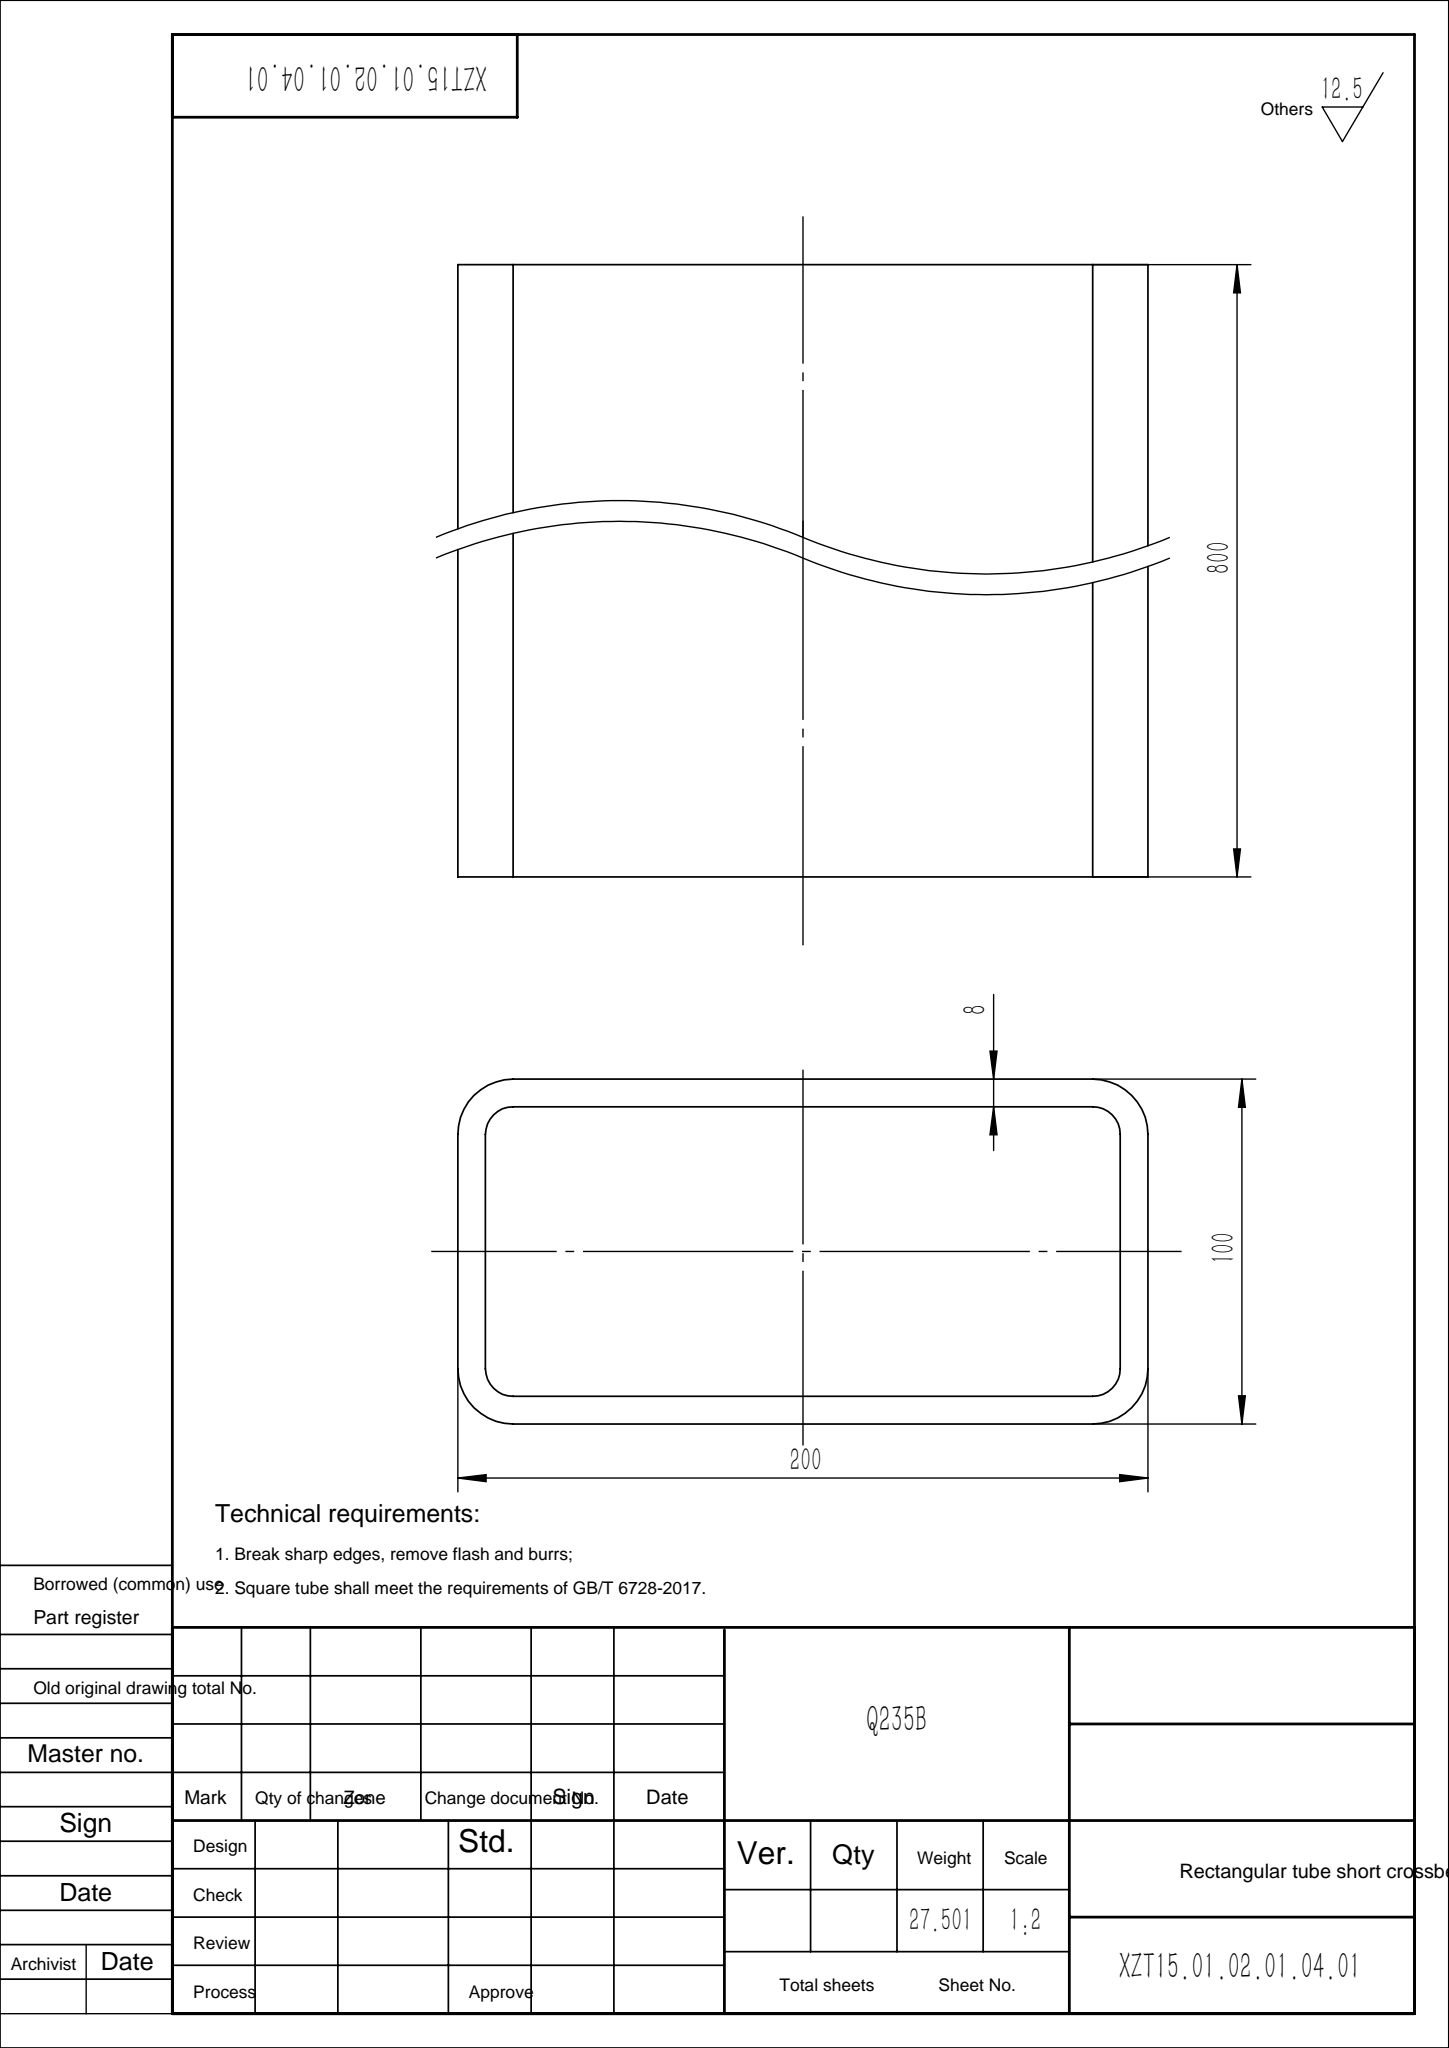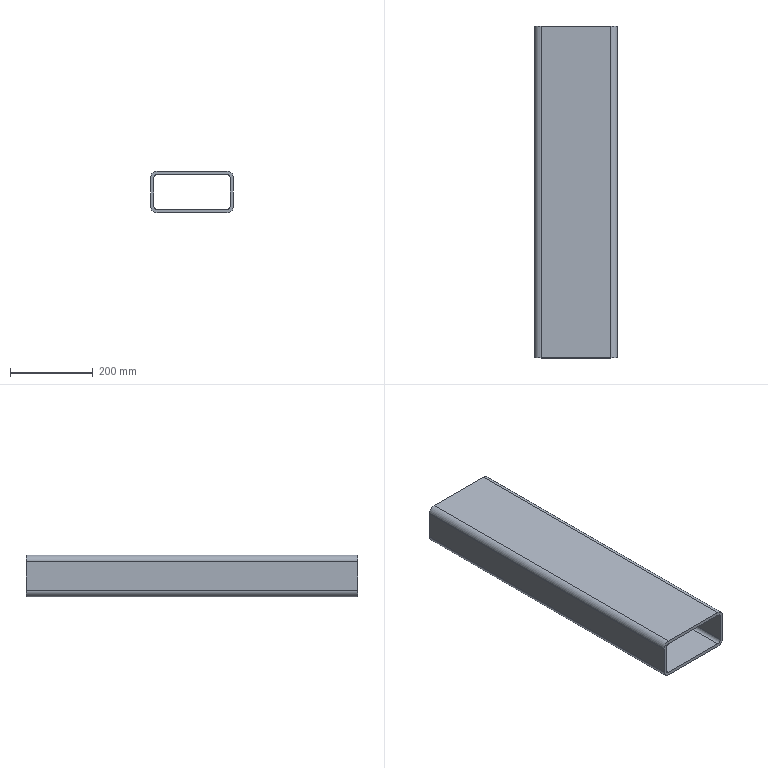Part | SolidWorks | features WeldMemberFeat 1, WeldmentFeature 1 | 1 solid | 18 faces | box 200 x 800 x 100 mm | volume 3503349 mm3 | plane 10 | cylinder 8 | commonest cylinder face diameters 16 x4 32 x4
STEP:
#1=CARTESIAN_POINT('',(84.,0.,50.));
#2=VERTEX_POINT('',#1);
#3=CARTESIAN_POINT('',(100.,0.,34.));
#4=VERTEX_POINT('',#3);
#5=CARTESIAN_POINT('',(84.,0.,34.));
#6=DIRECTION('',(0.,1.,0.));
#7=DIRECTION('',(0.,0.,1.));
#8=AXIS2_PLACEMENT_3D('',#5,#6,#7);
#9=CIRCLE('',#8,16.);
#10=EDGE_CURVE('',#2,#4,#9,.T.);
#11=ORIENTED_EDGE('',*,*,#10,.T.);
#12=CARTESIAN_POINT('',(100.,800.,34.));
#13=VERTEX_POINT('',#12);
#14=CARTESIAN_POINT('',(100.,800.,34.));
#15=DIRECTION('',(0.,-1.,0.));
#16=VECTOR('',#15,1000.);
#17=LINE('',#14,#16);
#18=EDGE_CURVE('',#13,#4,#17,.T.);
#19=ORIENTED_EDGE('',*,*,#18,.F.);
#20=CARTESIAN_POINT('',(84.,800.,50.));
#21=VERTEX_POINT('',#20);
#22=CARTESIAN_POINT('',(84.,800.,34.));
#23=DIRECTION('',(0.,1.,0.));
#24=DIRECTION('',(0.,0.,1.));
#25=AXIS2_PLACEMENT_3D('',#22,#23,#24);
#26=CIRCLE('',#25,16.);
#27=EDGE_CURVE('',#21,#13,#26,.T.);
#28=ORIENTED_EDGE('',*,*,#27,.F.);
#29=CARTESIAN_POINT('',(84.,800.,50.));
#30=DIRECTION('',(0.,-1.,0.));
#31=VECTOR('',#30,1000.);
#32=LINE('',#29,#31);
#33=EDGE_CURVE('',#21,#2,#32,.T.);
#34=ORIENTED_EDGE('',*,*,#33,.T.);
#35=EDGE_LOOP('',(#11,#19,#28,#34));
#36=FACE_OUTER_BOUND('',#35,.T.);
#37=CARTESIAN_POINT('',(84.,800.,34.));
#38=DIRECTION('',(0.,-1.,0.));
#39=DIRECTION('',(0.,0.,-1.));
#40=AXIS2_PLACEMENT_3D('',#37,#38,#39);
#41=CYLINDRICAL_SURFACE('',#40,16.);
#42=ADVANCED_FACE('',(#36),#41,.T.);
#43=CARTESIAN_POINT('',(100.,0.,-34.));
#44=VERTEX_POINT('',#43);
#45=CARTESIAN_POINT('',(100.,0.,34.));
#46=DIRECTION('',(0.,0.,-1.));
#47=VECTOR('',#46,1000.);
#48=LINE('',#45,#47);
#49=EDGE_CURVE('',#4,#44,#48,.T.);
#50=ORIENTED_EDGE('',*,*,#49,.T.);
#51=CARTESIAN_POINT('',(100.,800.,-34.));
#52=VERTEX_POINT('',#51);
#53=CARTESIAN_POINT('',(100.,800.,-34.));
#54=DIRECTION('',(0.,-1.,0.));
#55=VECTOR('',#54,1000.);
#56=LINE('',#53,#55);
#57=EDGE_CURVE('',#52,#44,#56,.T.);
#58=ORIENTED_EDGE('',*,*,#57,.F.);
#59=CARTESIAN_POINT('',(100.,800.,34.));
#60=DIRECTION('',(0.,0.,-1.));
#61=VECTOR('',#60,1000.);
#62=LINE('',#59,#61);
#63=EDGE_CURVE('',#13,#52,#62,.T.);
#64=ORIENTED_EDGE('',*,*,#63,.F.);
#65=ORIENTED_EDGE('',*,*,#18,.T.);
#66=EDGE_LOOP('',(#50,#58,#64,#65));
#67=FACE_OUTER_BOUND('',#66,.T.);
#68=CARTESIAN_POINT('',(100.,800.,34.));
#69=DIRECTION('',(-1.,0.,0.));
#70=DIRECTION('',(0.,0.,1.));
#71=AXIS2_PLACEMENT_3D('',#68,#69,#70);
#72=PLANE('',#71);
#73=ADVANCED_FACE('',(#67),#72,.F.);
#74=CARTESIAN_POINT('',(84.,0.,-50.));
#75=VERTEX_POINT('',#74);
#76=CARTESIAN_POINT('',(84.,0.,-34.));
#77=DIRECTION('',(0.,1.,0.));
#78=DIRECTION('',(0.,0.,1.));
#79=AXIS2_PLACEMENT_3D('',#76,#77,#78);
#80=CIRCLE('',#79,16.);
#81=EDGE_CURVE('',#44,#75,#80,.T.);
#82=ORIENTED_EDGE('',*,*,#81,.T.);
#83=CARTESIAN_POINT('',(84.,800.,-50.));
#84=VERTEX_POINT('',#83);
#85=CARTESIAN_POINT('',(84.,800.,-50.));
#86=DIRECTION('',(0.,-1.,0.));
#87=VECTOR('',#86,1000.);
#88=LINE('',#85,#87);
#89=EDGE_CURVE('',#84,#75,#88,.T.);
#90=ORIENTED_EDGE('',*,*,#89,.F.);
#91=CARTESIAN_POINT('',(84.,800.,-34.));
#92=DIRECTION('',(0.,1.,0.));
#93=DIRECTION('',(0.,0.,1.));
#94=AXIS2_PLACEMENT_3D('',#91,#92,#93);
#95=CIRCLE('',#94,16.);
#96=EDGE_CURVE('',#52,#84,#95,.T.);
#97=ORIENTED_EDGE('',*,*,#96,.F.);
#98=ORIENTED_EDGE('',*,*,#57,.T.);
#99=EDGE_LOOP('',(#82,#90,#97,#98));
#100=FACE_OUTER_BOUND('',#99,.T.);
#101=CARTESIAN_POINT('',(84.,800.,-34.));
#102=DIRECTION('',(0.,-1.,0.));
#103=DIRECTION('',(0.,0.,-1.));
#104=AXIS2_PLACEMENT_3D('',#101,#102,#103);
#105=CYLINDRICAL_SURFACE('',#104,16.);
#106=ADVANCED_FACE('',(#100),#105,.T.);
#107=CARTESIAN_POINT('',(-84.,0.,-50.));
#108=VERTEX_POINT('',#107);
#109=CARTESIAN_POINT('',(-84.,0.,-50.));
#110=DIRECTION('',(-1.,0.,0.));
#111=VECTOR('',#110,1000.);
#112=LINE('',#109,#111);
#113=EDGE_CURVE('',#75,#108,#112,.T.);
#114=ORIENTED_EDGE('',*,*,#113,.T.);
#115=CARTESIAN_POINT('',(-84.,800.,-50.));
#116=VERTEX_POINT('',#115);
#117=CARTESIAN_POINT('',(-84.,800.,-50.));
#118=DIRECTION('',(0.,-1.,0.));
#119=VECTOR('',#118,1000.);
#120=LINE('',#117,#119);
#121=EDGE_CURVE('',#116,#108,#120,.T.);
#122=ORIENTED_EDGE('',*,*,#121,.F.);
#123=CARTESIAN_POINT('',(-84.,800.,-50.));
#124=DIRECTION('',(-1.,0.,0.));
#125=VECTOR('',#124,1000.);
#126=LINE('',#123,#125);
#127=EDGE_CURVE('',#84,#116,#126,.T.);
#128=ORIENTED_EDGE('',*,*,#127,.F.);
#129=ORIENTED_EDGE('',*,*,#89,.T.);
#130=EDGE_LOOP('',(#114,#122,#128,#129));
#131=FACE_OUTER_BOUND('',#130,.T.);
#132=CARTESIAN_POINT('',(-84.,800.,-50.));
#133=DIRECTION('',(0.,0.,1.));
#134=DIRECTION('',(1.,0.,0.));
#135=AXIS2_PLACEMENT_3D('',#132,#133,#134);
#136=PLANE('',#135);
#137=ADVANCED_FACE('',(#131),#136,.F.);
#138=CARTESIAN_POINT('',(-100.,0.,-34.));
#139=VERTEX_POINT('',#138);
#140=CARTESIAN_POINT('',(-84.,0.,-34.));
#141=DIRECTION('',(0.,1.,0.));
#142=DIRECTION('',(0.,0.,1.));
#143=AXIS2_PLACEMENT_3D('',#140,#141,#142);
#144=CIRCLE('',#143,16.);
#145=EDGE_CURVE('',#108,#139,#144,.T.);
#146=ORIENTED_EDGE('',*,*,#145,.T.);
#147=CARTESIAN_POINT('',(-100.,800.,-34.));
#148=VERTEX_POINT('',#147);
#149=CARTESIAN_POINT('',(-100.,800.,-34.));
#150=DIRECTION('',(0.,-1.,0.));
#151=VECTOR('',#150,1000.);
#152=LINE('',#149,#151);
#153=EDGE_CURVE('',#148,#139,#152,.T.);
#154=ORIENTED_EDGE('',*,*,#153,.F.);
#155=CARTESIAN_POINT('',(-84.,800.,-34.));
#156=DIRECTION('',(0.,1.,0.));
#157=DIRECTION('',(0.,0.,1.));
#158=AXIS2_PLACEMENT_3D('',#155,#156,#157);
#159=CIRCLE('',#158,16.);
#160=EDGE_CURVE('',#116,#148,#159,.T.);
#161=ORIENTED_EDGE('',*,*,#160,.F.);
#162=ORIENTED_EDGE('',*,*,#121,.T.);
#163=EDGE_LOOP('',(#146,#154,#161,#162));
#164=FACE_OUTER_BOUND('',#163,.T.);
#165=CARTESIAN_POINT('',(-84.,800.,-34.));
#166=DIRECTION('',(0.,-1.,0.));
#167=DIRECTION('',(0.,0.,-1.));
#168=AXIS2_PLACEMENT_3D('',#165,#166,#167);
#169=CYLINDRICAL_SURFACE('',#168,16.);
#170=ADVANCED_FACE('',(#164),#169,.T.);
#171=CARTESIAN_POINT('',(-100.,0.,34.));
#172=VERTEX_POINT('',#171);
#173=CARTESIAN_POINT('',(-100.,0.,-34.));
#174=DIRECTION('',(0.,0.,1.));
#175=VECTOR('',#174,1000.);
#176=LINE('',#173,#175);
#177=EDGE_CURVE('',#139,#172,#176,.T.);
#178=ORIENTED_EDGE('',*,*,#177,.T.);
#179=CARTESIAN_POINT('',(-100.,800.,34.));
#180=VERTEX_POINT('',#179);
#181=CARTESIAN_POINT('',(-100.,800.,34.));
#182=DIRECTION('',(0.,-1.,0.));
#183=VECTOR('',#182,1000.);
#184=LINE('',#181,#183);
#185=EDGE_CURVE('',#180,#172,#184,.T.);
#186=ORIENTED_EDGE('',*,*,#185,.F.);
#187=CARTESIAN_POINT('',(-100.,800.,-34.));
#188=DIRECTION('',(0.,0.,1.));
#189=VECTOR('',#188,1000.);
#190=LINE('',#187,#189);
#191=EDGE_CURVE('',#148,#180,#190,.T.);
#192=ORIENTED_EDGE('',*,*,#191,.F.);
#193=ORIENTED_EDGE('',*,*,#153,.T.);
#194=EDGE_LOOP('',(#178,#186,#192,#193));
#195=FACE_OUTER_BOUND('',#194,.T.);
#196=CARTESIAN_POINT('',(-100.,800.,-34.));
#197=DIRECTION('',(1.,0.,0.));
#198=DIRECTION('',(0.,0.,-1.));
#199=AXIS2_PLACEMENT_3D('',#196,#197,#198);
#200=PLANE('',#199);
#201=ADVANCED_FACE('',(#195),#200,.F.);
#202=CARTESIAN_POINT('',(-84.,0.,50.));
#203=VERTEX_POINT('',#202);
#204=CARTESIAN_POINT('',(-84.,0.,34.));
#205=DIRECTION('',(0.,1.,0.));
#206=DIRECTION('',(0.,0.,1.));
#207=AXIS2_PLACEMENT_3D('',#204,#205,#206);
#208=CIRCLE('',#207,16.);
#209=EDGE_CURVE('',#172,#203,#208,.T.);
#210=ORIENTED_EDGE('',*,*,#209,.T.);
#211=CARTESIAN_POINT('',(-84.,800.,50.));
#212=VERTEX_POINT('',#211);
#213=CARTESIAN_POINT('',(-84.,800.,50.));
#214=DIRECTION('',(0.,-1.,0.));
#215=VECTOR('',#214,1000.);
#216=LINE('',#213,#215);
#217=EDGE_CURVE('',#212,#203,#216,.T.);
#218=ORIENTED_EDGE('',*,*,#217,.F.);
#219=CARTESIAN_POINT('',(-84.,800.,34.));
#220=DIRECTION('',(0.,1.,0.));
#221=DIRECTION('',(0.,0.,1.));
#222=AXIS2_PLACEMENT_3D('',#219,#220,#221);
#223=CIRCLE('',#222,16.);
#224=EDGE_CURVE('',#180,#212,#223,.T.);
#225=ORIENTED_EDGE('',*,*,#224,.F.);
#226=ORIENTED_EDGE('',*,*,#185,.T.);
#227=EDGE_LOOP('',(#210,#218,#225,#226));
#228=FACE_OUTER_BOUND('',#227,.T.);
#229=CARTESIAN_POINT('',(-84.,800.,34.));
#230=DIRECTION('',(0.,-1.,0.));
#231=DIRECTION('',(0.,0.,-1.));
#232=AXIS2_PLACEMENT_3D('',#229,#230,#231);
#233=CYLINDRICAL_SURFACE('',#232,16.);
#234=ADVANCED_FACE('',(#228),#233,.T.);
#235=CARTESIAN_POINT('',(92.,0.,-34.));
#236=VERTEX_POINT('',#235);
#237=CARTESIAN_POINT('',(84.,0.,-42.));
#238=VERTEX_POINT('',#237);
#239=CARTESIAN_POINT('',(84.,0.,-34.));
#240=DIRECTION('',(0.,1.,0.));
#241=DIRECTION('',(0.,0.,1.));
#242=AXIS2_PLACEMENT_3D('',#239,#240,#241);
#243=CIRCLE('',#242,8.);
#244=EDGE_CURVE('',#236,#238,#243,.T.);
#245=ORIENTED_EDGE('',*,*,#244,.F.);
#246=CARTESIAN_POINT('',(92.,800.,-34.));
#247=VERTEX_POINT('',#246);
#248=CARTESIAN_POINT('',(92.,800.,-34.));
#249=DIRECTION('',(0.,-1.,0.));
#250=VECTOR('',#249,1000.);
#251=LINE('',#248,#250);
#252=EDGE_CURVE('',#247,#236,#251,.T.);
#253=ORIENTED_EDGE('',*,*,#252,.F.);
#254=CARTESIAN_POINT('',(84.,800.,-42.));
#255=VERTEX_POINT('',#254);
#256=CARTESIAN_POINT('',(84.,800.,-34.));
#257=DIRECTION('',(0.,1.,0.));
#258=DIRECTION('',(0.,0.,1.));
#259=AXIS2_PLACEMENT_3D('',#256,#257,#258);
#260=CIRCLE('',#259,8.);
#261=EDGE_CURVE('',#247,#255,#260,.T.);
#262=ORIENTED_EDGE('',*,*,#261,.T.);
#263=CARTESIAN_POINT('',(84.,800.,-42.));
#264=DIRECTION('',(0.,-1.,0.));
#265=VECTOR('',#264,1000.);
#266=LINE('',#263,#265);
#267=EDGE_CURVE('',#255,#238,#266,.T.);
#268=ORIENTED_EDGE('',*,*,#267,.T.);
#269=EDGE_LOOP('',(#245,#253,#262,#268));
#270=FACE_OUTER_BOUND('',#269,.T.);
#271=CARTESIAN_POINT('',(84.,800.,-34.));
#272=DIRECTION('',(0.,-1.,0.));
#273=DIRECTION('',(0.,0.,-1.));
#274=AXIS2_PLACEMENT_3D('',#271,#272,#273);
#275=CYLINDRICAL_SURFACE('',#274,8.);
#276=ADVANCED_FACE('',(#270),#275,.F.);
#277=CARTESIAN_POINT('',(92.,0.,34.));
#278=VERTEX_POINT('',#277);
#279=CARTESIAN_POINT('',(92.,0.,34.));
#280=DIRECTION('',(0.,0.,-1.));
#281=VECTOR('',#280,1000.);
#282=LINE('',#279,#281);
#283=EDGE_CURVE('',#278,#236,#282,.T.);
#284=ORIENTED_EDGE('',*,*,#283,.F.);
#285=CARTESIAN_POINT('',(92.,800.,34.));
#286=VERTEX_POINT('',#285);
#287=CARTESIAN_POINT('',(92.,800.,34.));
#288=DIRECTION('',(0.,-1.,0.));
#289=VECTOR('',#288,1000.);
#290=LINE('',#287,#289);
#291=EDGE_CURVE('',#286,#278,#290,.T.);
#292=ORIENTED_EDGE('',*,*,#291,.F.);
#293=CARTESIAN_POINT('',(92.,800.,34.));
#294=DIRECTION('',(0.,0.,-1.));
#295=VECTOR('',#294,1000.);
#296=LINE('',#293,#295);
#297=EDGE_CURVE('',#286,#247,#296,.T.);
#298=ORIENTED_EDGE('',*,*,#297,.T.);
#299=ORIENTED_EDGE('',*,*,#252,.T.);
#300=EDGE_LOOP('',(#284,#292,#298,#299));
#301=FACE_OUTER_BOUND('',#300,.T.);
#302=CARTESIAN_POINT('',(92.,800.,34.));
#303=DIRECTION('',(-1.,0.,0.));
#304=DIRECTION('',(0.,0.,1.));
#305=AXIS2_PLACEMENT_3D('',#302,#303,#304);
#306=PLANE('',#305);
#307=ADVANCED_FACE('',(#301),#306,.T.);
#308=CARTESIAN_POINT('',(84.,0.,42.));
#309=VERTEX_POINT('',#308);
#310=CARTESIAN_POINT('',(84.,0.,34.));
#311=DIRECTION('',(0.,1.,0.));
#312=DIRECTION('',(0.,0.,1.));
#313=AXIS2_PLACEMENT_3D('',#310,#311,#312);
#314=CIRCLE('',#313,8.);
#315=EDGE_CURVE('',#309,#278,#314,.T.);
#316=ORIENTED_EDGE('',*,*,#315,.F.);
#317=CARTESIAN_POINT('',(84.,800.,42.));
#318=VERTEX_POINT('',#317);
#319=CARTESIAN_POINT('',(84.,800.,42.));
#320=DIRECTION('',(0.,-1.,0.));
#321=VECTOR('',#320,1000.);
#322=LINE('',#319,#321);
#323=EDGE_CURVE('',#318,#309,#322,.T.);
#324=ORIENTED_EDGE('',*,*,#323,.F.);
#325=CARTESIAN_POINT('',(84.,800.,34.));
#326=DIRECTION('',(0.,1.,0.));
#327=DIRECTION('',(0.,0.,1.));
#328=AXIS2_PLACEMENT_3D('',#325,#326,#327);
#329=CIRCLE('',#328,8.);
#330=EDGE_CURVE('',#318,#286,#329,.T.);
#331=ORIENTED_EDGE('',*,*,#330,.T.);
#332=ORIENTED_EDGE('',*,*,#291,.T.);
#333=EDGE_LOOP('',(#316,#324,#331,#332));
#334=FACE_OUTER_BOUND('',#333,.T.);
#335=CARTESIAN_POINT('',(84.,800.,34.));
#336=DIRECTION('',(0.,-1.,0.));
#337=DIRECTION('',(0.,0.,-1.));
#338=AXIS2_PLACEMENT_3D('',#335,#336,#337);
#339=CYLINDRICAL_SURFACE('',#338,8.);
#340=ADVANCED_FACE('',(#334),#339,.F.);
#341=CARTESIAN_POINT('',(-84.,0.,42.));
#342=VERTEX_POINT('',#341);
#343=CARTESIAN_POINT('',(84.,0.,42.));
#344=DIRECTION('',(1.,0.,0.));
#345=VECTOR('',#344,1000.);
#346=LINE('',#343,#345);
#347=EDGE_CURVE('',#342,#309,#346,.T.);
#348=ORIENTED_EDGE('',*,*,#347,.F.);
#349=CARTESIAN_POINT('',(-84.,800.,42.));
#350=VERTEX_POINT('',#349);
#351=CARTESIAN_POINT('',(-84.,800.,42.));
#352=DIRECTION('',(0.,-1.,0.));
#353=VECTOR('',#352,1000.);
#354=LINE('',#351,#353);
#355=EDGE_CURVE('',#350,#342,#354,.T.);
#356=ORIENTED_EDGE('',*,*,#355,.F.);
#357=CARTESIAN_POINT('',(84.,800.,42.));
#358=DIRECTION('',(1.,0.,0.));
#359=VECTOR('',#358,1000.);
#360=LINE('',#357,#359);
#361=EDGE_CURVE('',#350,#318,#360,.T.);
#362=ORIENTED_EDGE('',*,*,#361,.T.);
#363=ORIENTED_EDGE('',*,*,#323,.T.);
#364=EDGE_LOOP('',(#348,#356,#362,#363));
#365=FACE_OUTER_BOUND('',#364,.T.);
#366=CARTESIAN_POINT('',(84.,800.,42.));
#367=DIRECTION('',(0.,0.,-1.));
#368=DIRECTION('',(-1.,0.,0.));
#369=AXIS2_PLACEMENT_3D('',#366,#367,#368);
#370=PLANE('',#369);
#371=ADVANCED_FACE('',(#365),#370,.T.);
#372=CARTESIAN_POINT('',(-92.,0.,34.));
#373=VERTEX_POINT('',#372);
#374=CARTESIAN_POINT('',(-84.,0.,34.));
#375=DIRECTION('',(0.,1.,0.));
#376=DIRECTION('',(0.,0.,1.));
#377=AXIS2_PLACEMENT_3D('',#374,#375,#376);
#378=CIRCLE('',#377,8.);
#379=EDGE_CURVE('',#373,#342,#378,.T.);
#380=ORIENTED_EDGE('',*,*,#379,.F.);
#381=CARTESIAN_POINT('',(-92.,800.,34.));
#382=VERTEX_POINT('',#381);
#383=CARTESIAN_POINT('',(-92.,800.,34.));
#384=DIRECTION('',(0.,-1.,0.));
#385=VECTOR('',#384,1000.);
#386=LINE('',#383,#385);
#387=EDGE_CURVE('',#382,#373,#386,.T.);
#388=ORIENTED_EDGE('',*,*,#387,.F.);
#389=CARTESIAN_POINT('',(-84.,800.,34.));
#390=DIRECTION('',(0.,1.,0.));
#391=DIRECTION('',(0.,0.,1.));
#392=AXIS2_PLACEMENT_3D('',#389,#390,#391);
#393=CIRCLE('',#392,8.);
#394=EDGE_CURVE('',#382,#350,#393,.T.);
#395=ORIENTED_EDGE('',*,*,#394,.T.);
#396=ORIENTED_EDGE('',*,*,#355,.T.);
#397=EDGE_LOOP('',(#380,#388,#395,#396));
#398=FACE_OUTER_BOUND('',#397,.T.);
#399=CARTESIAN_POINT('',(-84.,800.,34.));
#400=DIRECTION('',(0.,-1.,0.));
#401=DIRECTION('',(0.,0.,-1.));
#402=AXIS2_PLACEMENT_3D('',#399,#400,#401);
#403=CYLINDRICAL_SURFACE('',#402,8.);
#404=ADVANCED_FACE('',(#398),#403,.F.);
#405=CARTESIAN_POINT('',(-92.,0.,-34.));
#406=VERTEX_POINT('',#405);
#407=CARTESIAN_POINT('',(-92.,0.,-34.));
#408=DIRECTION('',(0.,0.,1.));
#409=VECTOR('',#408,1000.);
#410=LINE('',#407,#409);
#411=EDGE_CURVE('',#406,#373,#410,.T.);
#412=ORIENTED_EDGE('',*,*,#411,.F.);
#413=CARTESIAN_POINT('',(-92.,800.,-34.));
#414=VERTEX_POINT('',#413);
#415=CARTESIAN_POINT('',(-92.,800.,-34.));
#416=DIRECTION('',(0.,-1.,0.));
#417=VECTOR('',#416,1000.);
#418=LINE('',#415,#417);
#419=EDGE_CURVE('',#414,#406,#418,.T.);
#420=ORIENTED_EDGE('',*,*,#419,.F.);
#421=CARTESIAN_POINT('',(-92.,800.,-34.));
#422=DIRECTION('',(0.,0.,1.));
#423=VECTOR('',#422,1000.);
#424=LINE('',#421,#423);
#425=EDGE_CURVE('',#414,#382,#424,.T.);
#426=ORIENTED_EDGE('',*,*,#425,.T.);
#427=ORIENTED_EDGE('',*,*,#387,.T.);
#428=EDGE_LOOP('',(#412,#420,#426,#427));
#429=FACE_OUTER_BOUND('',#428,.T.);
#430=CARTESIAN_POINT('',(-92.,800.,-34.));
#431=DIRECTION('',(1.,0.,0.));
#432=DIRECTION('',(0.,0.,-1.));
#433=AXIS2_PLACEMENT_3D('',#430,#431,#432);
#434=PLANE('',#433);
#435=ADVANCED_FACE('',(#429),#434,.T.);
#436=CARTESIAN_POINT('',(-84.,0.,-42.));
#437=VERTEX_POINT('',#436);
#438=CARTESIAN_POINT('',(-84.,0.,-34.));
#439=DIRECTION('',(0.,1.,0.));
#440=DIRECTION('',(0.,0.,1.));
#441=AXIS2_PLACEMENT_3D('',#438,#439,#440);
#442=CIRCLE('',#441,8.);
#443=EDGE_CURVE('',#437,#406,#442,.T.);
#444=ORIENTED_EDGE('',*,*,#443,.F.);
#445=CARTESIAN_POINT('',(-84.,800.,-42.));
#446=VERTEX_POINT('',#445);
#447=CARTESIAN_POINT('',(-84.,800.,-42.));
#448=DIRECTION('',(0.,-1.,0.));
#449=VECTOR('',#448,1000.);
#450=LINE('',#447,#449);
#451=EDGE_CURVE('',#446,#437,#450,.T.);
#452=ORIENTED_EDGE('',*,*,#451,.F.);
#453=CARTESIAN_POINT('',(-84.,800.,-34.));
#454=DIRECTION('',(0.,1.,0.));
#455=DIRECTION('',(0.,0.,1.));
#456=AXIS2_PLACEMENT_3D('',#453,#454,#455);
#457=CIRCLE('',#456,8.);
#458=EDGE_CURVE('',#446,#414,#457,.T.);
#459=ORIENTED_EDGE('',*,*,#458,.T.);
#460=ORIENTED_EDGE('',*,*,#419,.T.);
#461=EDGE_LOOP('',(#444,#452,#459,#460));
#462=FACE_OUTER_BOUND('',#461,.T.);
#463=CARTESIAN_POINT('',(-84.,800.,-34.));
#464=DIRECTION('',(0.,-1.,0.));
#465=DIRECTION('',(0.,0.,-1.));
#466=AXIS2_PLACEMENT_3D('',#463,#464,#465);
#467=CYLINDRICAL_SURFACE('',#466,8.);
#468=ADVANCED_FACE('',(#462),#467,.F.);
#469=CARTESIAN_POINT('',(-84.,0.,-42.));
#470=DIRECTION('',(-1.,0.,0.));
#471=VECTOR('',#470,1000.);
#472=LINE('',#469,#471);
#473=EDGE_CURVE('',#238,#437,#472,.T.);
#474=ORIENTED_EDGE('',*,*,#473,.F.);
#475=ORIENTED_EDGE('',*,*,#267,.F.);
#476=CARTESIAN_POINT('',(-84.,800.,-42.));
#477=DIRECTION('',(-1.,0.,0.));
#478=VECTOR('',#477,1000.);
#479=LINE('',#476,#478);
#480=EDGE_CURVE('',#255,#446,#479,.T.);
#481=ORIENTED_EDGE('',*,*,#480,.T.);
#482=ORIENTED_EDGE('',*,*,#451,.T.);
#483=EDGE_LOOP('',(#474,#475,#481,#482));
#484=FACE_OUTER_BOUND('',#483,.T.);
#485=CARTESIAN_POINT('',(-84.,800.,-42.));
#486=DIRECTION('',(0.,0.,1.));
#487=DIRECTION('',(1.,0.,0.));
#488=AXIS2_PLACEMENT_3D('',#485,#486,#487);
#489=PLANE('',#488);
#490=ADVANCED_FACE('',(#484),#489,.T.);
#491=CARTESIAN_POINT('',(84.,0.,50.));
#492=DIRECTION('',(1.,0.,0.));
#493=VECTOR('',#492,1000.);
#494=LINE('',#491,#493);
#495=EDGE_CURVE('',#203,#2,#494,.T.);
#496=ORIENTED_EDGE('',*,*,#495,.T.);
#497=ORIENTED_EDGE('',*,*,#33,.F.);
#498=CARTESIAN_POINT('',(84.,800.,50.));
#499=DIRECTION('',(1.,0.,0.));
#500=VECTOR('',#499,1000.);
#501=LINE('',#498,#500);
#502=EDGE_CURVE('',#212,#21,#501,.T.);
#503=ORIENTED_EDGE('',*,*,#502,.F.);
#504=ORIENTED_EDGE('',*,*,#217,.T.);
#505=EDGE_LOOP('',(#496,#497,#503,#504));
#506=FACE_OUTER_BOUND('',#505,.T.);
#507=CARTESIAN_POINT('',(84.,800.,50.));
#508=DIRECTION('',(0.,0.,-1.));
#509=DIRECTION('',(-1.,0.,0.));
#510=AXIS2_PLACEMENT_3D('',#507,#508,#509);
#511=PLANE('',#510);
#512=ADVANCED_FACE('',(#506),#511,.F.);
#513=ORIENTED_EDGE('',*,*,#261,.F.);
#514=ORIENTED_EDGE('',*,*,#297,.F.);
#515=ORIENTED_EDGE('',*,*,#330,.F.);
#516=ORIENTED_EDGE('',*,*,#361,.F.);
#517=ORIENTED_EDGE('',*,*,#394,.F.);
#518=ORIENTED_EDGE('',*,*,#425,.F.);
#519=ORIENTED_EDGE('',*,*,#458,.F.);
#520=ORIENTED_EDGE('',*,*,#480,.F.);
#521=EDGE_LOOP('',(#513,#514,#515,#516,#517,#518,#519,#520));
#522=FACE_BOUND('',#521,.T.);
#523=ORIENTED_EDGE('',*,*,#27,.T.);
#524=ORIENTED_EDGE('',*,*,#63,.T.);
#525=ORIENTED_EDGE('',*,*,#96,.T.);
#526=ORIENTED_EDGE('',*,*,#127,.T.);
#527=ORIENTED_EDGE('',*,*,#160,.T.);
#528=ORIENTED_EDGE('',*,*,#191,.T.);
#529=ORIENTED_EDGE('',*,*,#224,.T.);
#530=ORIENTED_EDGE('',*,*,#502,.T.);
#531=EDGE_LOOP('',(#523,#524,#525,#526,#527,#528,#529,#530));
#532=FACE_OUTER_BOUND('',#531,.T.);
#533=CARTESIAN_POINT('',(84.,800.,34.));
#534=DIRECTION('',(0.,1.,0.));
#535=DIRECTION('',(0.,0.,1.));
#536=AXIS2_PLACEMENT_3D('',#533,#534,#535);
#537=PLANE('',#536);
#538=ADVANCED_FACE('',(#522,#532),#537,.T.);
#539=ORIENTED_EDGE('',*,*,#244,.T.);
#540=ORIENTED_EDGE('',*,*,#473,.T.);
#541=ORIENTED_EDGE('',*,*,#443,.T.);
#542=ORIENTED_EDGE('',*,*,#411,.T.);
#543=ORIENTED_EDGE('',*,*,#379,.T.);
#544=ORIENTED_EDGE('',*,*,#347,.T.);
#545=ORIENTED_EDGE('',*,*,#315,.T.);
#546=ORIENTED_EDGE('',*,*,#283,.T.);
#547=EDGE_LOOP('',(#539,#540,#541,#542,#543,#544,#545,#546));
#548=FACE_BOUND('',#547,.T.);
#549=ORIENTED_EDGE('',*,*,#10,.F.);
#550=ORIENTED_EDGE('',*,*,#495,.F.);
#551=ORIENTED_EDGE('',*,*,#209,.F.);
#552=ORIENTED_EDGE('',*,*,#177,.F.);
#553=ORIENTED_EDGE('',*,*,#145,.F.);
#554=ORIENTED_EDGE('',*,*,#113,.F.);
#555=ORIENTED_EDGE('',*,*,#81,.F.);
#556=ORIENTED_EDGE('',*,*,#49,.F.);
#557=EDGE_LOOP('',(#549,#550,#551,#552,#553,#554,#555,#556));
#558=FACE_OUTER_BOUND('',#557,.T.);
#559=CARTESIAN_POINT('',(84.,0.,34.));
#560=DIRECTION('',(0.,1.,0.));
#561=DIRECTION('',(0.,0.,1.));
#562=AXIS2_PLACEMENT_3D('',#559,#560,#561);
#563=PLANE('',#562);
#564=ADVANCED_FACE('',(#548,#558),#563,.F.);
#565=CLOSED_SHELL('',(#42,#73,#106,#137,#170,#201,#234,#276,#307,#340,#371,#404,#435,#468,#490,#512,#538,#564));
#566=MANIFOLD_SOLID_BREP('',#565);
#567=CARTESIAN_POINT('',(0.,0.,0.));
#568=DIRECTION('',(0.,0.,1.));
#569=DIRECTION('',(1.,0.,0.));
#570=AXIS2_PLACEMENT_3D('',#567,#568,#569);
#571=(LENGTH_UNIT()NAMED_UNIT(*)SI_UNIT(.MILLI.,.METRE.));
#572=UNCERTAINTY_MEASURE_WITH_UNIT(LENGTH_MEASURE(0.00001),#571,'','');
#573=(NAMED_UNIT(*)PLANE_ANGLE_UNIT()SI_UNIT($,.RADIAN.));
#574=(NAMED_UNIT(*)SI_UNIT($,.STERADIAN.)SOLID_ANGLE_UNIT());
#575=(GEOMETRIC_REPRESENTATION_CONTEXT(3)GLOBAL_UNCERTAINTY_ASSIGNED_CONTEXT((#572))GLOBAL_UNIT_ASSIGNED_CONTEXT((#571,#573,#574))REPRESENTATION_CONTEXT('',''));
#576=ADVANCED_BREP_SHAPE_REPRESENTATION('',(#566,#570),#575);